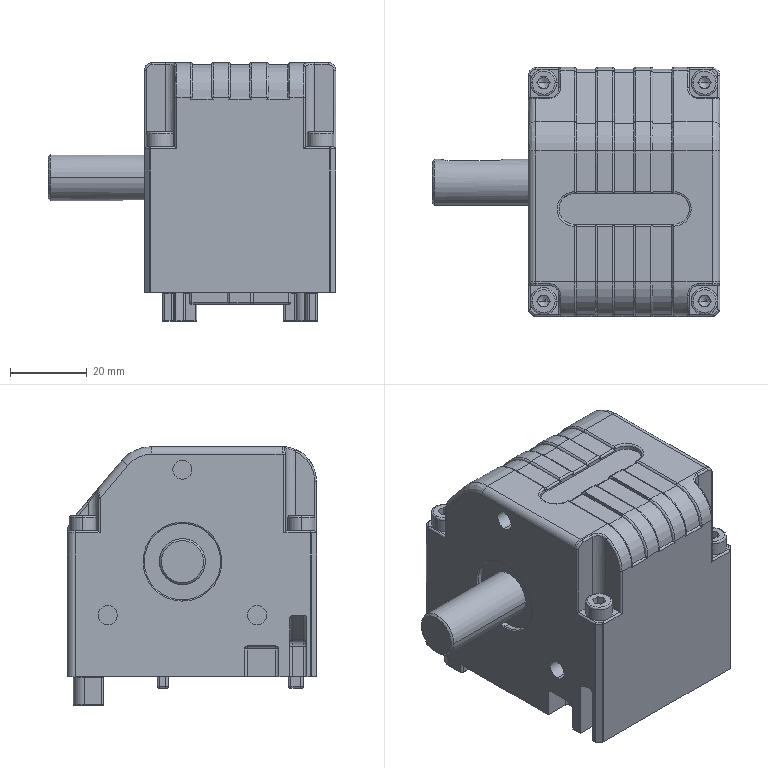Part | STEP file | Copy of K50-right output shaft^K50A-1H20-S(formula driven)-L700-motor left- | 6 solids | 716 faces | box 75.1 x 65 x 67.5 mm | volume 175722 mm3 | cylinder 294 | plane 209 | spline 187 | cone 26 | commonest cylinder face diameters 1 x85 5 x38 0.4 x24 4 x22 1.6 x18 0.6 x12